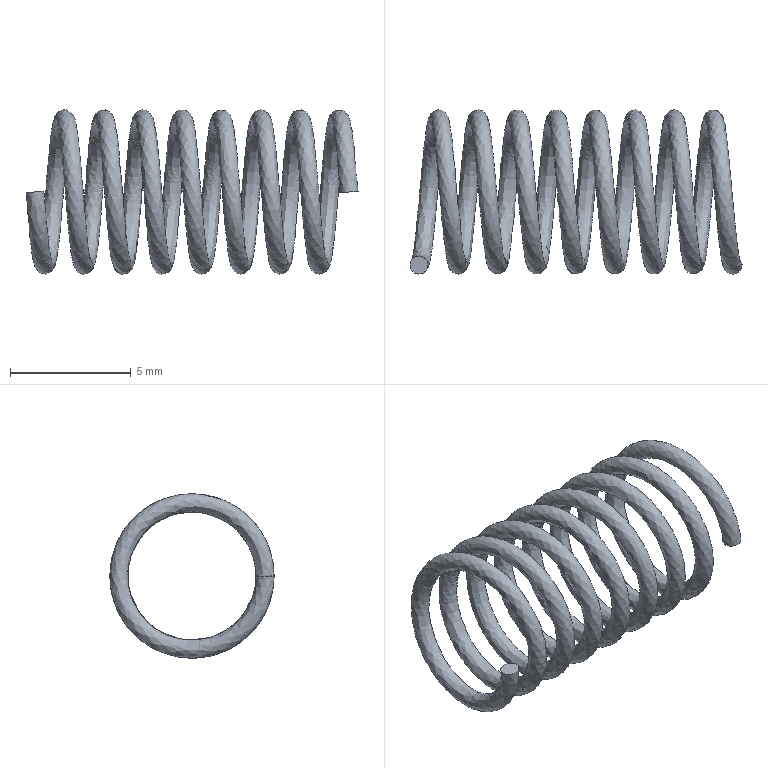Part | STEP file | 1-29.3 | 1 solid | 3 faces | box 13.747 x 6.8 x 6.802 mm | volume 67.319 mm3 | plane 2 | spline 1